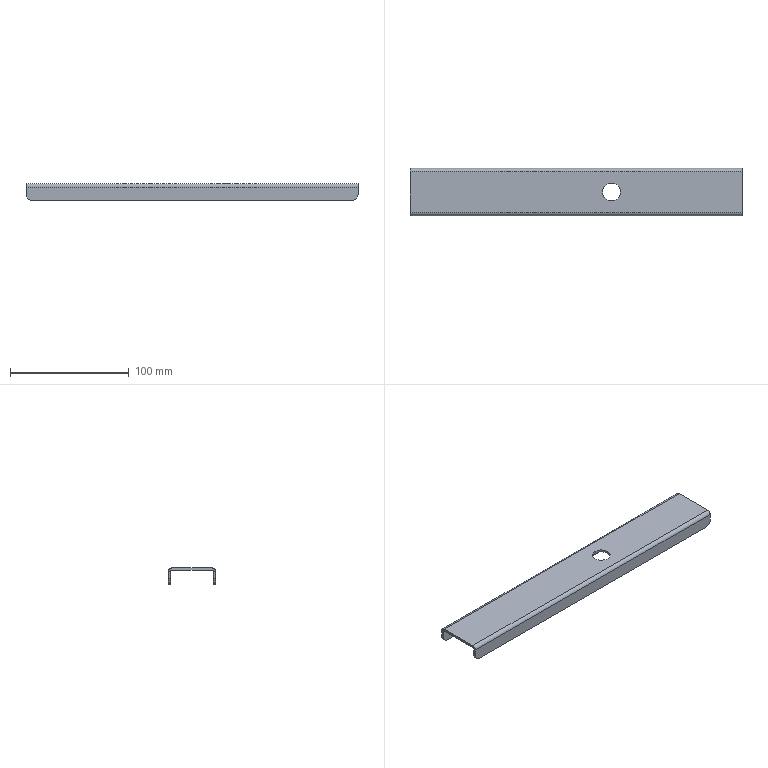Part | SolidWorks | features BaseBody 1 | 1 solid | 28 faces | box 280 x 40 x 14 mm | volume 34482 mm3 | plane 18 | cylinder 10 | commonest cylinder face diameters 10 x4 2 x2 6 x2 15 x2
STEP:
#1=CARTESIAN_POINT('',(-135.,20.,-14.));
#2=VERTEX_POINT('',#1);
#3=CARTESIAN_POINT('',(-140.,20.,-9.));
#4=VERTEX_POINT('',#3);
#5=CARTESIAN_POINT('',(-135.,20.,-9.));
#6=DIRECTION('',(0.,1.,0.));
#7=DIRECTION('',(0.,0.,1.));
#8=AXIS2_PLACEMENT_3D('',#5,#6,#7);
#9=CIRCLE('',#8,5.);
#10=EDGE_CURVE('',#2,#4,#9,.T.);
#11=ORIENTED_EDGE('',*,*,#10,.F.);
#12=CARTESIAN_POINT('',(-135.,18.,-14.));
#13=VERTEX_POINT('',#12);
#14=CARTESIAN_POINT('',(-135.,20.,-14.));
#15=DIRECTION('',(0.,1.,0.));
#16=VECTOR('',#15,1000.);
#17=LINE('',#14,#16);
#18=EDGE_CURVE('',#13,#2,#17,.T.);
#19=ORIENTED_EDGE('',*,*,#18,.F.);
#20=CARTESIAN_POINT('',(-140.,18.,-9.));
#21=VERTEX_POINT('',#20);
#22=CARTESIAN_POINT('',(-135.,18.,-9.));
#23=DIRECTION('',(0.,-1.,0.));
#24=DIRECTION('',(0.,0.,1.));
#25=AXIS2_PLACEMENT_3D('',#22,#23,#24);
#26=CIRCLE('',#25,5.);
#27=EDGE_CURVE('',#21,#13,#26,.T.);
#28=ORIENTED_EDGE('',*,*,#27,.F.);
#29=CARTESIAN_POINT('',(-140.,20.,-9.));
#30=DIRECTION('',(0.,-1.,0.));
#31=VECTOR('',#30,1000.);
#32=LINE('',#29,#31);
#33=EDGE_CURVE('',#4,#21,#32,.T.);
#34=ORIENTED_EDGE('',*,*,#33,.F.);
#35=EDGE_LOOP('',(#11,#19,#28,#34));
#36=FACE_OUTER_BOUND('',#35,.T.);
#37=CARTESIAN_POINT('',(-135.,20.,-9.));
#38=DIRECTION('',(0.,-1.,0.));
#39=DIRECTION('',(0.,0.,-1.));
#40=AXIS2_PLACEMENT_3D('',#37,#38,#39);
#41=CYLINDRICAL_SURFACE('',#40,5.);
#42=ADVANCED_FACE('',(#36),#41,.T.);
#43=CARTESIAN_POINT('',(-140.,-20.,-9.));
#44=VERTEX_POINT('',#43);
#45=CARTESIAN_POINT('',(-135.,-20.,-14.));
#46=VERTEX_POINT('',#45);
#47=CARTESIAN_POINT('',(-135.,-20.,-9.));
#48=DIRECTION('',(0.,-1.,0.));
#49=DIRECTION('',(0.,0.,1.));
#50=AXIS2_PLACEMENT_3D('',#47,#48,#49);
#51=CIRCLE('',#50,5.);
#52=EDGE_CURVE('',#44,#46,#51,.T.);
#53=ORIENTED_EDGE('',*,*,#52,.F.);
#54=CARTESIAN_POINT('',(-140.,-18.,-9.));
#55=VERTEX_POINT('',#54);
#56=CARTESIAN_POINT('',(-140.,-20.,-9.));
#57=DIRECTION('',(0.,-1.,0.));
#58=VECTOR('',#57,1000.);
#59=LINE('',#56,#58);
#60=EDGE_CURVE('',#55,#44,#59,.T.);
#61=ORIENTED_EDGE('',*,*,#60,.F.);
#62=CARTESIAN_POINT('',(-135.,-18.,-14.));
#63=VERTEX_POINT('',#62);
#64=CARTESIAN_POINT('',(-135.,-18.,-9.));
#65=DIRECTION('',(0.,1.,0.));
#66=DIRECTION('',(0.,0.,1.));
#67=AXIS2_PLACEMENT_3D('',#64,#65,#66);
#68=CIRCLE('',#67,5.);
#69=EDGE_CURVE('',#63,#55,#68,.T.);
#70=ORIENTED_EDGE('',*,*,#69,.F.);
#71=CARTESIAN_POINT('',(-135.,-20.,-14.));
#72=DIRECTION('',(0.,1.,0.));
#73=VECTOR('',#72,1000.);
#74=LINE('',#71,#73);
#75=EDGE_CURVE('',#46,#63,#74,.T.);
#76=ORIENTED_EDGE('',*,*,#75,.F.);
#77=EDGE_LOOP('',(#53,#61,#70,#76));
#78=FACE_OUTER_BOUND('',#77,.T.);
#79=CARTESIAN_POINT('',(-135.,-20.,-9.));
#80=DIRECTION('',(0.,1.,0.));
#81=DIRECTION('',(0.,0.,1.));
#82=AXIS2_PLACEMENT_3D('',#79,#80,#81);
#83=CYLINDRICAL_SURFACE('',#82,5.);
#84=ADVANCED_FACE('',(#78),#83,.T.);
#85=CARTESIAN_POINT('',(135.,-20.,-14.));
#86=VERTEX_POINT('',#85);
#87=CARTESIAN_POINT('',(140.,-20.,-9.));
#88=VERTEX_POINT('',#87);
#89=CARTESIAN_POINT('',(135.,-20.,-9.));
#90=DIRECTION('',(0.,-1.,0.));
#91=DIRECTION('',(0.,0.,1.));
#92=AXIS2_PLACEMENT_3D('',#89,#90,#91);
#93=CIRCLE('',#92,5.);
#94=EDGE_CURVE('',#86,#88,#93,.T.);
#95=ORIENTED_EDGE('',*,*,#94,.F.);
#96=CARTESIAN_POINT('',(135.,-18.,-14.));
#97=VERTEX_POINT('',#96);
#98=CARTESIAN_POINT('',(135.,-20.,-14.));
#99=DIRECTION('',(0.,-1.,0.));
#100=VECTOR('',#99,1000.);
#101=LINE('',#98,#100);
#102=EDGE_CURVE('',#97,#86,#101,.T.);
#103=ORIENTED_EDGE('',*,*,#102,.F.);
#104=CARTESIAN_POINT('',(140.,-18.,-9.));
#105=VERTEX_POINT('',#104);
#106=CARTESIAN_POINT('',(135.,-18.,-9.));
#107=DIRECTION('',(0.,1.,0.));
#108=DIRECTION('',(0.,0.,1.));
#109=AXIS2_PLACEMENT_3D('',#106,#107,#108);
#110=CIRCLE('',#109,5.);
#111=EDGE_CURVE('',#105,#97,#110,.T.);
#112=ORIENTED_EDGE('',*,*,#111,.F.);
#113=CARTESIAN_POINT('',(140.,-20.,-9.));
#114=DIRECTION('',(0.,1.,0.));
#115=VECTOR('',#114,1000.);
#116=LINE('',#113,#115);
#117=EDGE_CURVE('',#88,#105,#116,.T.);
#118=ORIENTED_EDGE('',*,*,#117,.F.);
#119=EDGE_LOOP('',(#95,#103,#112,#118));
#120=FACE_OUTER_BOUND('',#119,.T.);
#121=CARTESIAN_POINT('',(135.,-20.,-9.));
#122=DIRECTION('',(0.,1.,0.));
#123=DIRECTION('',(0.,0.,1.));
#124=AXIS2_PLACEMENT_3D('',#121,#122,#123);
#125=CYLINDRICAL_SURFACE('',#124,5.);
#126=ADVANCED_FACE('',(#120),#125,.T.);
#127=CARTESIAN_POINT('',(140.,20.,-9.));
#128=VERTEX_POINT('',#127);
#129=CARTESIAN_POINT('',(135.,20.,-14.));
#130=VERTEX_POINT('',#129);
#131=CARTESIAN_POINT('',(135.,20.,-9.));
#132=DIRECTION('',(0.,1.,0.));
#133=DIRECTION('',(0.,0.,1.));
#134=AXIS2_PLACEMENT_3D('',#131,#132,#133);
#135=CIRCLE('',#134,5.);
#136=EDGE_CURVE('',#128,#130,#135,.T.);
#137=ORIENTED_EDGE('',*,*,#136,.F.);
#138=CARTESIAN_POINT('',(140.,18.,-9.));
#139=VERTEX_POINT('',#138);
#140=CARTESIAN_POINT('',(140.,20.,-9.));
#141=DIRECTION('',(0.,1.,0.));
#142=VECTOR('',#141,1000.);
#143=LINE('',#140,#142);
#144=EDGE_CURVE('',#139,#128,#143,.T.);
#145=ORIENTED_EDGE('',*,*,#144,.F.);
#146=CARTESIAN_POINT('',(135.,18.,-14.));
#147=VERTEX_POINT('',#146);
#148=CARTESIAN_POINT('',(135.,18.,-9.));
#149=DIRECTION('',(0.,-1.,0.));
#150=DIRECTION('',(0.,0.,1.));
#151=AXIS2_PLACEMENT_3D('',#148,#149,#150);
#152=CIRCLE('',#151,5.);
#153=EDGE_CURVE('',#147,#139,#152,.T.);
#154=ORIENTED_EDGE('',*,*,#153,.F.);
#155=CARTESIAN_POINT('',(135.,20.,-14.));
#156=DIRECTION('',(0.,-1.,0.));
#157=VECTOR('',#156,1000.);
#158=LINE('',#155,#157);
#159=EDGE_CURVE('',#130,#147,#158,.T.);
#160=ORIENTED_EDGE('',*,*,#159,.F.);
#161=EDGE_LOOP('',(#137,#145,#154,#160));
#162=FACE_OUTER_BOUND('',#161,.T.);
#163=CARTESIAN_POINT('',(135.,20.,-9.));
#164=DIRECTION('',(0.,-1.,0.));
#165=DIRECTION('',(0.,0.,-1.));
#166=AXIS2_PLACEMENT_3D('',#163,#164,#165);
#167=CYLINDRICAL_SURFACE('',#166,5.);
#168=ADVANCED_FACE('',(#162),#167,.T.);
#169=CARTESIAN_POINT('',(0.,-18.,-14.));
#170=DIRECTION('',(-1.,0.,0.));
#171=VECTOR('',#170,1000.);
#172=LINE('',#169,#171);
#173=EDGE_CURVE('',#97,#63,#172,.T.);
#174=ORIENTED_EDGE('',*,*,#173,.F.);
#175=ORIENTED_EDGE('',*,*,#102,.T.);
#176=CARTESIAN_POINT('',(140.,-20.,-14.));
#177=DIRECTION('',(-1.,0.,0.));
#178=VECTOR('',#177,1000.);
#179=LINE('',#176,#178);
#180=EDGE_CURVE('',#86,#46,#179,.T.);
#181=ORIENTED_EDGE('',*,*,#180,.T.);
#182=ORIENTED_EDGE('',*,*,#75,.T.);
#183=EDGE_LOOP('',(#174,#175,#181,#182));
#184=FACE_OUTER_BOUND('',#183,.T.);
#185=CARTESIAN_POINT('',(140.,-20.,-14.));
#186=DIRECTION('',(0.,0.,-1.));
#187=DIRECTION('',(0.,-1.,0.));
#188=AXIS2_PLACEMENT_3D('',#185,#186,#187);
#189=PLANE('',#188);
#190=ADVANCED_FACE('',(#184),#189,.T.);
#191=CARTESIAN_POINT('',(140.,-18.,-3.));
#192=VERTEX_POINT('',#191);
#193=CARTESIAN_POINT('',(140.,-18.,0.));
#194=DIRECTION('',(0.,0.,-1.));
#195=VECTOR('',#194,1000.);
#196=LINE('',#193,#195);
#197=EDGE_CURVE('',#192,#105,#196,.T.);
#198=ORIENTED_EDGE('',*,*,#197,.T.);
#199=ORIENTED_EDGE('',*,*,#111,.T.);
#200=ORIENTED_EDGE('',*,*,#173,.T.);
#201=ORIENTED_EDGE('',*,*,#69,.T.);
#202=CARTESIAN_POINT('',(-140.,-18.,-3.));
#203=VERTEX_POINT('',#202);
#204=CARTESIAN_POINT('',(-140.,-18.,0.));
#205=DIRECTION('',(0.,0.,1.));
#206=VECTOR('',#205,1000.);
#207=LINE('',#204,#206);
#208=EDGE_CURVE('',#55,#203,#207,.T.);
#209=ORIENTED_EDGE('',*,*,#208,.T.);
#210=CARTESIAN_POINT('',(140.,-18.,-3.));
#211=DIRECTION('',(-1.,0.,0.));
#212=VECTOR('',#211,1000.);
#213=LINE('',#210,#212);
#214=EDGE_CURVE('',#192,#203,#213,.T.);
#215=ORIENTED_EDGE('',*,*,#214,.F.);
#216=EDGE_LOOP('',(#198,#199,#200,#201,#209,#215));
#217=FACE_OUTER_BOUND('',#216,.T.);
#218=CARTESIAN_POINT('',(0.,-18.,0.));
#219=DIRECTION('',(0.,1.,0.));
#220=DIRECTION('',(0.,0.,-1.));
#221=AXIS2_PLACEMENT_3D('',#218,#219,#220);
#222=PLANE('',#221);
#223=ADVANCED_FACE('',(#217),#222,.T.);
#224=ORIENTED_EDGE('',*,*,#180,.F.);
#225=ORIENTED_EDGE('',*,*,#94,.T.);
#226=CARTESIAN_POINT('',(140.,-20.,-3.));
#227=VERTEX_POINT('',#226);
#228=CARTESIAN_POINT('',(140.,-20.,-2.));
#229=DIRECTION('',(0.,0.,-1.));
#230=VECTOR('',#229,1000.);
#231=LINE('',#228,#230);
#232=EDGE_CURVE('',#227,#88,#231,.T.);
#233=ORIENTED_EDGE('',*,*,#232,.F.);
#234=CARTESIAN_POINT('',(-140.,-20.,-3.));
#235=VERTEX_POINT('',#234);
#236=CARTESIAN_POINT('',(140.,-20.,-3.));
#237=DIRECTION('',(1.,0.,0.));
#238=VECTOR('',#237,1000.);
#239=LINE('',#236,#238);
#240=EDGE_CURVE('',#235,#227,#239,.T.);
#241=ORIENTED_EDGE('',*,*,#240,.F.);
#242=CARTESIAN_POINT('',(-140.,-20.,-14.));
#243=DIRECTION('',(0.,0.,1.));
#244=VECTOR('',#243,1000.);
#245=LINE('',#242,#244);
#246=EDGE_CURVE('',#44,#235,#245,.T.);
#247=ORIENTED_EDGE('',*,*,#246,.F.);
#248=ORIENTED_EDGE('',*,*,#52,.T.);
#249=EDGE_LOOP('',(#224,#225,#233,#241,#247,#248));
#250=FACE_OUTER_BOUND('',#249,.T.);
#251=CARTESIAN_POINT('',(0.,-20.,0.));
#252=DIRECTION('',(0.,1.,0.));
#253=DIRECTION('',(0.,0.,-1.));
#254=AXIS2_PLACEMENT_3D('',#251,#252,#253);
#255=PLANE('',#254);
#256=ADVANCED_FACE('',(#250),#255,.F.);
#257=ORIENTED_EDGE('',*,*,#208,.F.);
#258=ORIENTED_EDGE('',*,*,#60,.T.);
#259=ORIENTED_EDGE('',*,*,#246,.T.);
#260=CARTESIAN_POINT('',(-140.,-18.,-3.));
#261=DIRECTION('',(0.,-1.,0.));
#262=VECTOR('',#261,1000.);
#263=LINE('',#260,#262);
#264=EDGE_CURVE('',#203,#235,#263,.T.);
#265=ORIENTED_EDGE('',*,*,#264,.F.);
#266=EDGE_LOOP('',(#257,#258,#259,#265));
#267=FACE_OUTER_BOUND('',#266,.T.);
#268=CARTESIAN_POINT('',(-140.,-20.,-14.));
#269=DIRECTION('',(-1.,0.,0.));
#270=DIRECTION('',(0.,0.,1.));
#271=AXIS2_PLACEMENT_3D('',#268,#269,#270);
#272=PLANE('',#271);
#273=ADVANCED_FACE('',(#267),#272,.T.);
#274=ORIENTED_EDGE('',*,*,#232,.T.);
#275=ORIENTED_EDGE('',*,*,#117,.T.);
#276=ORIENTED_EDGE('',*,*,#197,.F.);
#277=CARTESIAN_POINT('',(140.,-20.,-3.));
#278=DIRECTION('',(0.,-1.,0.));
#279=VECTOR('',#278,1000.);
#280=LINE('',#277,#279);
#281=EDGE_CURVE('',#192,#227,#280,.T.);
#282=ORIENTED_EDGE('',*,*,#281,.T.);
#283=EDGE_LOOP('',(#274,#275,#276,#282));
#284=FACE_OUTER_BOUND('',#283,.T.);
#285=CARTESIAN_POINT('',(140.,-20.,-2.));
#286=DIRECTION('',(1.,0.,0.));
#287=DIRECTION('',(0.,1.,0.));
#288=AXIS2_PLACEMENT_3D('',#285,#286,#287);
#289=PLANE('',#288);
#290=ADVANCED_FACE('',(#284),#289,.T.);
#291=CARTESIAN_POINT('',(-140.,-17.,-2.));
#292=VERTEX_POINT('',#291);
#293=CARTESIAN_POINT('',(140.,-17.,-2.));
#294=VERTEX_POINT('',#293);
#295=CARTESIAN_POINT('',(-140.,-17.,-2.));
#296=DIRECTION('',(1.,0.,0.));
#297=VECTOR('',#296,1000.);
#298=LINE('',#295,#297);
#299=EDGE_CURVE('',#292,#294,#298,.T.);
#300=ORIENTED_EDGE('',*,*,#299,.T.);
#301=CARTESIAN_POINT('',(140.,-17.,-3.));
#302=DIRECTION('',(1.,0.,0.));
#303=DIRECTION('',(0.,0.,1.));
#304=AXIS2_PLACEMENT_3D('',#301,#302,#303);
#305=CIRCLE('',#304,1.);
#306=EDGE_CURVE('',#294,#192,#305,.T.);
#307=ORIENTED_EDGE('',*,*,#306,.T.);
#308=ORIENTED_EDGE('',*,*,#214,.T.);
#309=CARTESIAN_POINT('',(-140.,-17.,-3.));
#310=DIRECTION('',(-1.,0.,0.));
#311=DIRECTION('',(0.,0.,1.));
#312=AXIS2_PLACEMENT_3D('',#309,#310,#311);
#313=CIRCLE('',#312,1.);
#314=EDGE_CURVE('',#203,#292,#313,.T.);
#315=ORIENTED_EDGE('',*,*,#314,.T.);
#316=EDGE_LOOP('',(#300,#307,#308,#315));
#317=FACE_OUTER_BOUND('',#316,.T.);
#318=CARTESIAN_POINT('',(-140.,-17.,-3.));
#319=DIRECTION('',(-1.,0.,0.));
#320=DIRECTION('',(0.,-1.,0.));
#321=AXIS2_PLACEMENT_3D('',#318,#319,#320);
#322=CYLINDRICAL_SURFACE('',#321,1.);
#323=ADVANCED_FACE('',(#317),#322,.F.);
#324=CARTESIAN_POINT('',(-140.,-17.,0.));
#325=VERTEX_POINT('',#324);
#326=CARTESIAN_POINT('',(140.,-17.,0.));
#327=VERTEX_POINT('',#326);
#328=CARTESIAN_POINT('',(-140.,-17.,0.));
#329=DIRECTION('',(1.,0.,0.));
#330=VECTOR('',#329,1000.);
#331=LINE('',#328,#330);
#332=EDGE_CURVE('',#325,#327,#331,.T.);
#333=ORIENTED_EDGE('',*,*,#332,.F.);
#334=CARTESIAN_POINT('',(-140.,-17.,-3.));
#335=DIRECTION('',(-1.,0.,0.));
#336=DIRECTION('',(0.,0.,1.));
#337=AXIS2_PLACEMENT_3D('',#334,#335,#336);
#338=CIRCLE('',#337,3.);
#339=EDGE_CURVE('',#235,#325,#338,.T.);
#340=ORIENTED_EDGE('',*,*,#339,.F.);
#341=ORIENTED_EDGE('',*,*,#240,.T.);
#342=CARTESIAN_POINT('',(140.,-17.,-3.));
#343=DIRECTION('',(1.,0.,0.));
#344=DIRECTION('',(0.,0.,1.));
#345=AXIS2_PLACEMENT_3D('',#342,#343,#344);
#346=CIRCLE('',#345,3.);
#347=EDGE_CURVE('',#327,#227,#346,.T.);
#348=ORIENTED_EDGE('',*,*,#347,.F.);
#349=EDGE_LOOP('',(#333,#340,#341,#348));
#350=FACE_OUTER_BOUND('',#349,.T.);
#351=CARTESIAN_POINT('',(-140.,-17.,-3.));
#352=DIRECTION('',(-1.,0.,0.));
#353=DIRECTION('',(0.,-1.,0.));
#354=AXIS2_PLACEMENT_3D('',#351,#352,#353);
#355=CYLINDRICAL_SURFACE('',#354,3.);
#356=ADVANCED_FACE('',(#350),#355,.T.);
#357=ORIENTED_EDGE('',*,*,#314,.F.);
#358=ORIENTED_EDGE('',*,*,#264,.T.);
#359=ORIENTED_EDGE('',*,*,#339,.T.);
#360=CARTESIAN_POINT('',(-140.,-17.,-2.));
#361=DIRECTION('',(0.,0.,1.));
#362=VECTOR('',#361,1000.);
#363=LINE('',#360,#362);
#364=EDGE_CURVE('',#292,#325,#363,.T.);
#365=ORIENTED_EDGE('',*,*,#364,.F.);
#366=EDGE_LOOP('',(#357,#358,#359,#365));
#367=FACE_OUTER_BOUND('',#366,.T.);
#368=CARTESIAN_POINT('',(-140.,-17.,-3.));
#369=DIRECTION('',(1.,0.,0.));
#370=DIRECTION('',(0.,1.,0.));
#371=AXIS2_PLACEMENT_3D('',#368,#369,#370);
#372=PLANE('',#371);
#373=ADVANCED_FACE('',(#367),#372,.F.);
#374=ORIENTED_EDGE('',*,*,#281,.F.);
#375=ORIENTED_EDGE('',*,*,#306,.F.);
#376=CARTESIAN_POINT('',(140.,-17.,-2.));
#377=DIRECTION('',(0.,0.,1.));
#378=VECTOR('',#377,1000.);
#379=LINE('',#376,#378);
#380=EDGE_CURVE('',#294,#327,#379,.T.);
#381=ORIENTED_EDGE('',*,*,#380,.T.);
#382=ORIENTED_EDGE('',*,*,#347,.T.);
#383=EDGE_LOOP('',(#374,#375,#381,#382));
#384=FACE_OUTER_BOUND('',#383,.T.);
#385=CARTESIAN_POINT('',(140.,-17.,-3.));
#386=DIRECTION('',(1.,0.,0.));
#387=DIRECTION('',(0.,1.,0.));
#388=AXIS2_PLACEMENT_3D('',#385,#386,#387);
#389=PLANE('',#388);
#390=ADVANCED_FACE('',(#384),#389,.T.);
#391=CARTESIAN_POINT('',(140.,20.,-14.));
#392=DIRECTION('',(1.,0.,0.));
#393=VECTOR('',#392,1000.);
#394=LINE('',#391,#393);
#395=EDGE_CURVE('',#2,#130,#394,.T.);
#396=ORIENTED_EDGE('',*,*,#395,.T.);
#397=ORIENTED_EDGE('',*,*,#159,.T.);
#398=CARTESIAN_POINT('',(0.,18.,-14.));
#399=DIRECTION('',(1.,0.,0.));
#400=VECTOR('',#399,1000.);
#401=LINE('',#398,#400);
#402=EDGE_CURVE('',#13,#147,#401,.T.);
#403=ORIENTED_EDGE('',*,*,#402,.F.);
#404=ORIENTED_EDGE('',*,*,#18,.T.);
#405=EDGE_LOOP('',(#396,#397,#403,#404));
#406=FACE_OUTER_BOUND('',#405,.T.);
#407=CARTESIAN_POINT('',(140.,20.,-14.));
#408=DIRECTION('',(0.,0.,-1.));
#409=DIRECTION('',(-1.,0.,0.));
#410=AXIS2_PLACEMENT_3D('',#407,#408,#409);
#411=PLANE('',#410);
#412=ADVANCED_FACE('',(#406),#411,.T.);
#413=ORIENTED_EDGE('',*,*,#402,.T.);
#414=ORIENTED_EDGE('',*,*,#153,.T.);
#415=CARTESIAN_POINT('',(140.,18.,-3.));
#416=VERTEX_POINT('',#415);
#417=CARTESIAN_POINT('',(140.,18.,0.));
#418=DIRECTION('',(0.,0.,1.));
#419=VECTOR('',#418,1000.);
#420=LINE('',#417,#419);
#421=EDGE_CURVE('',#139,#416,#420,.T.);
#422=ORIENTED_EDGE('',*,*,#421,.T.);
#423=CARTESIAN_POINT('',(-140.,18.,-3.));
#424=VERTEX_POINT('',#423);
#425=CARTESIAN_POINT('',(-140.,18.,-3.));
#426=DIRECTION('',(1.,0.,0.));
#427=VECTOR('',#426,1000.);
#428=LINE('',#425,#427);
#429=EDGE_CURVE('',#424,#416,#428,.T.);
#430=ORIENTED_EDGE('',*,*,#429,.F.);
#431=CARTESIAN_POINT('',(-140.,18.,0.));
#432=DIRECTION('',(0.,0.,-1.));
#433=VECTOR('',#432,1000.);
#434=LINE('',#431,#433);
#435=EDGE_CURVE('',#424,#21,#434,.T.);
#436=ORIENTED_EDGE('',*,*,#435,.T.);
#437=ORIENTED_EDGE('',*,*,#27,.T.);
#438=EDGE_LOOP('',(#413,#414,#422,#430,#436,#437));
#439=FACE_OUTER_BOUND('',#438,.T.);
#440=CARTESIAN_POINT('',(0.,18.,0.));
#441=DIRECTION('',(0.,1.,0.));
#442=DIRECTION('',(0.,0.,-1.));
#443=AXIS2_PLACEMENT_3D('',#440,#441,#442);
#444=PLANE('',#443);
#445=ADVANCED_FACE('',(#439),#444,.F.);
#446=CARTESIAN_POINT('',(140.,20.,-3.));
#447=VERTEX_POINT('',#446);
#448=CARTESIAN_POINT('',(140.,20.,-2.));
#449=DIRECTION('',(0.,0.,1.));
#450=VECTOR('',#449,1000.);
#451=LINE('',#448,#450);
#452=EDGE_CURVE('',#128,#447,#451,.T.);
#453=ORIENTED_EDGE('',*,*,#452,.F.);
#454=ORIENTED_EDGE('',*,*,#136,.T.);
#455=ORIENTED_EDGE('',*,*,#395,.F.);
#456=ORIENTED_EDGE('',*,*,#10,.T.);
#457=CARTESIAN_POINT('',(-140.,20.,-3.));
#458=VERTEX_POINT('',#457);
#459=CARTESIAN_POINT('',(-140.,20.,-14.));
#460=DIRECTION('',(0.,0.,-1.));
#461=VECTOR('',#460,1000.);
#462=LINE('',#459,#461);
#463=EDGE_CURVE('',#458,#4,#462,.T.);
#464=ORIENTED_EDGE('',*,*,#463,.F.);
#465=CARTESIAN_POINT('',(0.,20.,-3.));
#466=DIRECTION('',(1.,0.,0.));
#467=VECTOR('',#466,1000.);
#468=LINE('',#465,#467);
#469=EDGE_CURVE('',#458,#447,#468,.T.);
#470=ORIENTED_EDGE('',*,*,#469,.T.);
#471=EDGE_LOOP('',(#453,#454,#455,#456,#464,#470));
#472=FACE_OUTER_BOUND('',#471,.T.);
#473=CARTESIAN_POINT('',(0.,20.,0.));
#474=DIRECTION('',(0.,1.,0.));
#475=DIRECTION('',(0.,0.,-1.));
#476=AXIS2_PLACEMENT_3D('',#473,#474,#475);
#477=PLANE('',#476);
#478=ADVANCED_FACE('',(#472),#477,.T.);
#479=ORIENTED_EDGE('',*,*,#463,.T.);
#480=ORIENTED_EDGE('',*,*,#33,.T.);
#481=ORIENTED_EDGE('',*,*,#435,.F.);
#482=CARTESIAN_POINT('',(-140.,20.,-3.));
#483=DIRECTION('',(0.,1.,0.));
#484=VECTOR('',#483,1000.);
#485=LINE('',#482,#484);
#486=EDGE_CURVE('',#424,#458,#485,.T.);
#487=ORIENTED_EDGE('',*,*,#486,.T.);
#488=EDGE_LOOP('',(#479,#480,#481,#487));
#489=FACE_OUTER_BOUND('',#488,.T.);
#490=CARTESIAN_POINT('',(-140.,20.,-14.));
#491=DIRECTION('',(-1.,0.,0.));
#492=DIRECTION('',(0.,0.,1.));
#493=AXIS2_PLACEMENT_3D('',#490,#491,#492);
#494=PLANE('',#493);
#495=ADVANCED_FACE('',(#489),#494,.T.);
#496=ORIENTED_EDGE('',*,*,#421,.F.);
#497=ORIENTED_EDGE('',*,*,#144,.T.);
#498=ORIENTED_EDGE('',*,*,#452,.T.);
#499=CARTESIAN_POINT('',(140.,18.,-3.));
#500=DIRECTION('',(0.,1.,0.));
#501=VECTOR('',#500,1000.);
#502=LINE('',#499,#501);
#503=EDGE_CURVE('',#416,#447,#502,.T.);
#504=ORIENTED_EDGE('',*,*,#503,.F.);
#505=EDGE_LOOP('',(#496,#497,#498,#504));
#506=FACE_OUTER_BOUND('',#505,.T.);
#507=CARTESIAN_POINT('',(140.,20.,-2.));
#508=DIRECTION('',(1.,0.,0.));
#509=DIRECTION('',(0.,1.,0.));
#510=AXIS2_PLACEMENT_3D('',#507,#508,#509);
#511=PLANE('',#510);
#512=ADVANCED_FACE('',(#506),#511,.T.);
#513=CARTESIAN_POINT('',(140.,17.,-2.));
#514=VERTEX_POINT('',#513);
#515=CARTESIAN_POINT('',(-140.,17.,-2.));
#516=VERTEX_POINT('',#515);
#517=CARTESIAN_POINT('',(140.,17.,-2.));
#518=DIRECTION('',(-1.,0.,0.));
#519=VECTOR('',#518,1000.);
#520=LINE('',#517,#519);
#521=EDGE_CURVE('',#514,#516,#520,.T.);
#522=ORIENTED_EDGE('',*,*,#521,.T.);
#523=CARTESIAN_POINT('',(-140.,17.,-3.));
#524=DIRECTION('',(-1.,0.,0.));
#525=DIRECTION('',(0.,0.,-1.));
#526=AXIS2_PLACEMENT_3D('',#523,#524,#525);
#527=CIRCLE('',#526,1.);
#528=EDGE_CURVE('',#516,#424,#527,.T.);
#529=ORIENTED_EDGE('',*,*,#528,.T.);
#530=ORIENTED_EDGE('',*,*,#429,.T.);
#531=CARTESIAN_POINT('',(140.,17.,-3.));
#532=DIRECTION('',(1.,0.,0.));
#533=DIRECTION('',(0.,0.,-1.));
#534=AXIS2_PLACEMENT_3D('',#531,#532,#533);
#535=CIRCLE('',#534,1.);
#536=EDGE_CURVE('',#416,#514,#535,.T.);
#537=ORIENTED_EDGE('',*,*,#536,.T.);
#538=EDGE_LOOP('',(#522,#529,#530,#537));
#539=FACE_OUTER_BOUND('',#538,.T.);
#540=CARTESIAN_POINT('',(140.,17.,-3.));
#541=DIRECTION('',(1.,0.,0.));
#542=DIRECTION('',(0.,1.,0.));
#543=AXIS2_PLACEMENT_3D('',#540,#541,#542);
#544=CYLINDRICAL_SURFACE('',#543,1.);
#545=ADVANCED_FACE('',(#539),#544,.F.);
#546=CARTESIAN_POINT('',(140.,17.,0.));
#547=VERTEX_POINT('',#546);
#548=CARTESIAN_POINT('',(-140.,17.,0.));
#549=VERTEX_POINT('',#548);
#550=CARTESIAN_POINT('',(140.,17.,0.));
#551=DIRECTION('',(-1.,0.,0.));
#552=VECTOR('',#551,1000.);
#553=LINE('',#550,#552);
#554=EDGE_CURVE('',#547,#549,#553,.T.);
#555=ORIENTED_EDGE('',*,*,#554,.F.);
#556=CARTESIAN_POINT('',(140.,17.,-3.));
#557=DIRECTION('',(1.,0.,0.));
#558=DIRECTION('',(0.,0.,-1.));
#559=AXIS2_PLACEMENT_3D('',#556,#557,#558);
#560=CIRCLE('',#559,3.);
#561=EDGE_CURVE('',#447,#547,#560,.T.);
#562=ORIENTED_EDGE('',*,*,#561,.F.);
#563=ORIENTED_EDGE('',*,*,#469,.F.);
#564=CARTESIAN_POINT('',(-140.,17.,-3.));
#565=DIRECTION('',(-1.,0.,0.));
#566=DIRECTION('',(0.,0.,-1.));
#567=AXIS2_PLACEMENT_3D('',#564,#565,#566);
#568=CIRCLE('',#567,3.);
#569=EDGE_CURVE('',#549,#458,#568,.T.);
#570=ORIENTED_EDGE('',*,*,#569,.F.);
#571=EDGE_LOOP('',(#555,#562,#563,#570));
#572=FACE_OUTER_BOUND('',#571,.T.);
#573=CARTESIAN_POINT('',(140.,17.,-3.));
#574=DIRECTION('',(1.,0.,0.));
#575=DIRECTION('',(0.,1.,0.));
#576=AXIS2_PLACEMENT_3D('',#573,#574,#575);
#577=CYLINDRICAL_SURFACE('',#576,3.);
#578=ADVANCED_FACE('',(#572),#577,.T.);
#579=ORIENTED_EDGE('',*,*,#536,.F.);
#580=ORIENTED_EDGE('',*,*,#503,.T.);
#581=ORIENTED_EDGE('',*,*,#561,.T.);
#582=CARTESIAN_POINT('',(140.,17.,-2.));
#583=DIRECTION('',(0.,0.,1.));
#584=VECTOR('',#583,1000.);
#585=LINE('',#582,#584);
#586=EDGE_CURVE('',#514,#547,#585,.T.);
#587=ORIENTED_EDGE('',*,*,#586,.F.);
#588=EDGE_LOOP('',(#579,#580,#581,#587));
#589=FACE_OUTER_BOUND('',#588,.T.);
#590=CARTESIAN_POINT('',(140.,17.,-3.));
#591=DIRECTION('',(-1.,0.,0.));
#592=DIRECTION('',(0.,0.,1.));
#593=AXIS2_PLACEMENT_3D('',#590,#591,#592);
#594=PLANE('',#593);
#595=ADVANCED_FACE('',(#589),#594,.F.);
#596=ORIENTED_EDGE('',*,*,#486,.F.);
#597=ORIENTED_EDGE('',*,*,#528,.F.);
#598=CARTESIAN_POINT('',(-140.,17.,-2.));
#599=DIRECTION('',(0.,0.,1.));
#600=VECTOR('',#599,1000.);
#601=LINE('',#598,#600);
#602=EDGE_CURVE('',#516,#549,#601,.T.);
#603=ORIENTED_EDGE('',*,*,#602,.T.);
#604=ORIENTED_EDGE('',*,*,#569,.T.);
#605=EDGE_LOOP('',(#596,#597,#603,#604));
#606=FACE_OUTER_BOUND('',#605,.T.);
#607=CARTESIAN_POINT('',(-140.,17.,-3.));
#608=DIRECTION('',(-1.,0.,0.));
#609=DIRECTION('',(0.,0.,1.));
#610=AXIS2_PLACEMENT_3D('',#607,#608,#609);
#611=PLANE('',#610);
#612=ADVANCED_FACE('',(#606),#611,.T.);
#613=CARTESIAN_POINT('',(22.5,0.,-2.));
#614=VERTEX_POINT('',#613);
#615=CARTESIAN_POINT('',(22.5,0.,0.));
#616=VERTEX_POINT('',#615);
#617=CARTESIAN_POINT('',(22.5,0.,-10.));
#618=DIRECTION('',(0.,0.,1.));
#619=VECTOR('',#618,1000.);
#620=LINE('',#617,#619);
#621=EDGE_CURVE('',#614,#616,#620,.T.);
#622=ORIENTED_EDGE('',*,*,#621,.F.);
#623=CARTESIAN_POINT('',(37.5,0.,-2.));
#624=VERTEX_POINT('',#623);
#625=CARTESIAN_POINT('',(30.,0.,-2.));
#626=DIRECTION('',(0.,0.,-1.));
#627=DIRECTION('',(-1.,0.,0.));
#628=AXIS2_PLACEMENT_3D('',#625,#626,#627);
#629=CIRCLE('',#628,7.5);
#630=EDGE_CURVE('',#614,#624,#629,.T.);
#631=ORIENTED_EDGE('',*,*,#630,.T.);
#632=CARTESIAN_POINT('',(37.5,0.,0.));
#633=VERTEX_POINT('',#632);
#634=CARTESIAN_POINT('',(37.5,0.,-10.));
#635=DIRECTION('',(0.,0.,1.));
#636=VECTOR('',#635,1000.);
#637=LINE('',#634,#636);
#638=EDGE_CURVE('',#624,#633,#637,.T.);
#639=ORIENTED_EDGE('',*,*,#638,.T.);
#640=CARTESIAN_POINT('',(30.,0.,0.));
#641=DIRECTION('',(0.,0.,1.));
#642=DIRECTION('',(1.,0.,0.));
#643=AXIS2_PLACEMENT_3D('',#640,#641,#642);
#644=CIRCLE('',#643,7.5);
#645=EDGE_CURVE('',#633,#616,#644,.T.);
#646=ORIENTED_EDGE('',*,*,#645,.T.);
#647=EDGE_LOOP('',(#622,#631,#639,#646));
#648=FACE_OUTER_BOUND('',#647,.T.);
#649=CARTESIAN_POINT('',(30.,0.,-10.));
#650=DIRECTION('',(0.,0.,1.));
#651=DIRECTION('',(1.,0.,0.));
#652=AXIS2_PLACEMENT_3D('',#649,#650,#651);
#653=CYLINDRICAL_SURFACE('',#652,7.5);
#654=ADVANCED_FACE('',(#648),#653,.F.);
#655=ORIENTED_EDGE('',*,*,#380,.F.);
#656=CARTESIAN_POINT('',(140.,-20.,-2.));
#657=DIRECTION('',(0.,1.,0.));
#658=VECTOR('',#657,1000.);
#659=LINE('',#656,#658);
#660=EDGE_CURVE('',#294,#514,#659,.T.);
#661=ORIENTED_EDGE('',*,*,#660,.T.);
#662=ORIENTED_EDGE('',*,*,#586,.T.);
#663=CARTESIAN_POINT('',(140.,-20.,0.));
#664=DIRECTION('',(0.,1.,0.));
#665=VECTOR('',#664,1000.);
#666=LINE('',#663,#665);
#667=EDGE_CURVE('',#327,#547,#666,.T.);
#668=ORIENTED_EDGE('',*,*,#667,.F.);
#669=EDGE_LOOP('',(#655,#661,#662,#668));
#670=FACE_OUTER_BOUND('',#669,.T.);
#671=CARTESIAN_POINT('',(140.,-20.,-2.));
#672=DIRECTION('',(1.,0.,0.));
#673=DIRECTION('',(0.,1.,0.));
#674=AXIS2_PLACEMENT_3D('',#671,#672,#673);
#675=PLANE('',#674);
#676=ADVANCED_FACE('',(#670),#675,.T.);
#677=CARTESIAN_POINT('',(-140.,-20.,-2.));
#678=DIRECTION('',(0.,-1.,0.));
#679=VECTOR('',#678,1000.);
#680=LINE('',#677,#679);
#681=EDGE_CURVE('',#516,#292,#680,.T.);
#682=ORIENTED_EDGE('',*,*,#681,.T.);
#683=ORIENTED_EDGE('',*,*,#364,.T.);
#684=CARTESIAN_POINT('',(-140.,-20.,0.));
#685=DIRECTION('',(0.,-1.,0.));
#686=VECTOR('',#685,1000.);
#687=LINE('',#684,#686);
#688=EDGE_CURVE('',#549,#325,#687,.T.);
#689=ORIENTED_EDGE('',*,*,#688,.F.);
#690=ORIENTED_EDGE('',*,*,#602,.F.);
#691=EDGE_LOOP('',(#682,#683,#689,#690));
#692=FACE_OUTER_BOUND('',#691,.T.);
#693=CARTESIAN_POINT('',(-140.,-20.,-2.));
#694=DIRECTION('',(-1.,0.,0.));
#695=DIRECTION('',(0.,0.,1.));
#696=AXIS2_PLACEMENT_3D('',#693,#694,#695);
#697=PLANE('',#696);
#698=ADVANCED_FACE('',(#692),#697,.T.);
#699=ORIENTED_EDGE('',*,*,#645,.F.);
#700=CARTESIAN_POINT('',(30.,0.,0.));
#701=DIRECTION('',(0.,0.,1.));
#702=DIRECTION('',(1.,0.,0.));
#703=AXIS2_PLACEMENT_3D('',#700,#701,#702);
#704=CIRCLE('',#703,7.5);
#705=EDGE_CURVE('',#616,#633,#704,.T.);
#706=ORIENTED_EDGE('',*,*,#705,.F.);
#707=EDGE_LOOP('',(#699,#706));
#708=FACE_BOUND('',#707,.T.);
#709=ORIENTED_EDGE('',*,*,#332,.T.);
#710=ORIENTED_EDGE('',*,*,#667,.T.);
#711=ORIENTED_EDGE('',*,*,#554,.T.);
#712=ORIENTED_EDGE('',*,*,#688,.T.);
#713=EDGE_LOOP('',(#709,#710,#711,#712));
#714=FACE_OUTER_BOUND('',#713,.T.);
#715=CARTESIAN_POINT('',(0.,0.,0.));
#716=DIRECTION('',(0.,0.,-1.));
#717=DIRECTION('',(0.,-1.,0.));
#718=AXIS2_PLACEMENT_3D('',#715,#716,#717);
#719=PLANE('',#718);
#720=ADVANCED_FACE('',(#708,#714),#719,.F.);
#721=CARTESIAN_POINT('',(30.,0.,-2.));
#722=DIRECTION('',(0.,0.,-1.));
#723=DIRECTION('',(-1.,0.,0.));
#724=AXIS2_PLACEMENT_3D('',#721,#722,#723);
#725=CIRCLE('',#724,7.5);
#726=EDGE_CURVE('',#624,#614,#725,.T.);
#727=ORIENTED_EDGE('',*,*,#726,.F.);
#728=ORIENTED_EDGE('',*,*,#630,.F.);
#729=EDGE_LOOP('',(#727,#728));
#730=FACE_BOUND('',#729,.T.);
#731=ORIENTED_EDGE('',*,*,#660,.F.);
#732=ORIENTED_EDGE('',*,*,#299,.F.);
#733=ORIENTED_EDGE('',*,*,#681,.F.);
#734=ORIENTED_EDGE('',*,*,#521,.F.);
#735=EDGE_LOOP('',(#731,#732,#733,#734));
#736=FACE_OUTER_BOUND('',#735,.T.);
#737=CARTESIAN_POINT('',(0.,0.,-2.));
#738=DIRECTION('',(0.,0.,-1.));
#739=DIRECTION('',(0.,-1.,0.));
#740=AXIS2_PLACEMENT_3D('',#737,#738,#739);
#741=PLANE('',#740);
#742=ADVANCED_FACE('',(#730,#736),#741,.T.);
#743=ORIENTED_EDGE('',*,*,#726,.T.);
#744=ORIENTED_EDGE('',*,*,#621,.T.);
#745=ORIENTED_EDGE('',*,*,#705,.T.);
#746=ORIENTED_EDGE('',*,*,#638,.F.);
#747=EDGE_LOOP('',(#743,#744,#745,#746));
#748=FACE_OUTER_BOUND('',#747,.T.);
#749=CARTESIAN_POINT('',(30.,0.,-10.));
#750=DIRECTION('',(0.,0.,1.));
#751=DIRECTION('',(1.,0.,0.));
#752=AXIS2_PLACEMENT_3D('',#749,#750,#751);
#753=CYLINDRICAL_SURFACE('',#752,7.5);
#754=ADVANCED_FACE('',(#748),#753,.F.);
#755=CLOSED_SHELL('',(#42,#84,#126,#168,#190,#223,#256,#273,#290,#323,#356,#373,#390,#412,#445,#478,#495,#512,#545,#578,#595,#612,#654,#676,#698,#720,#742,#754));
#756=MANIFOLD_SOLID_BREP('',#755);
#757=CARTESIAN_POINT('',(0.,0.,0.));
#758=DIRECTION('',(0.,0.,1.));
#759=DIRECTION('',(1.,0.,0.));
#760=AXIS2_PLACEMENT_3D('',#757,#758,#759);
#761=(LENGTH_UNIT()NAMED_UNIT(*)SI_UNIT(.MILLI.,.METRE.));
#762=UNCERTAINTY_MEASURE_WITH_UNIT(LENGTH_MEASURE(0.00001),#761,'','');
#763=(NAMED_UNIT(*)PLANE_ANGLE_UNIT()SI_UNIT($,.RADIAN.));
#764=(NAMED_UNIT(*)SI_UNIT($,.STERADIAN.)SOLID_ANGLE_UNIT());
#765=(GEOMETRIC_REPRESENTATION_CONTEXT(3)GLOBAL_UNCERTAINTY_ASSIGNED_CONTEXT((#762))GLOBAL_UNIT_ASSIGNED_CONTEXT((#761,#763,#764))REPRESENTATION_CONTEXT('',''));
#766=ADVANCED_BREP_SHAPE_REPRESENTATION('',(#756,#760),#765);